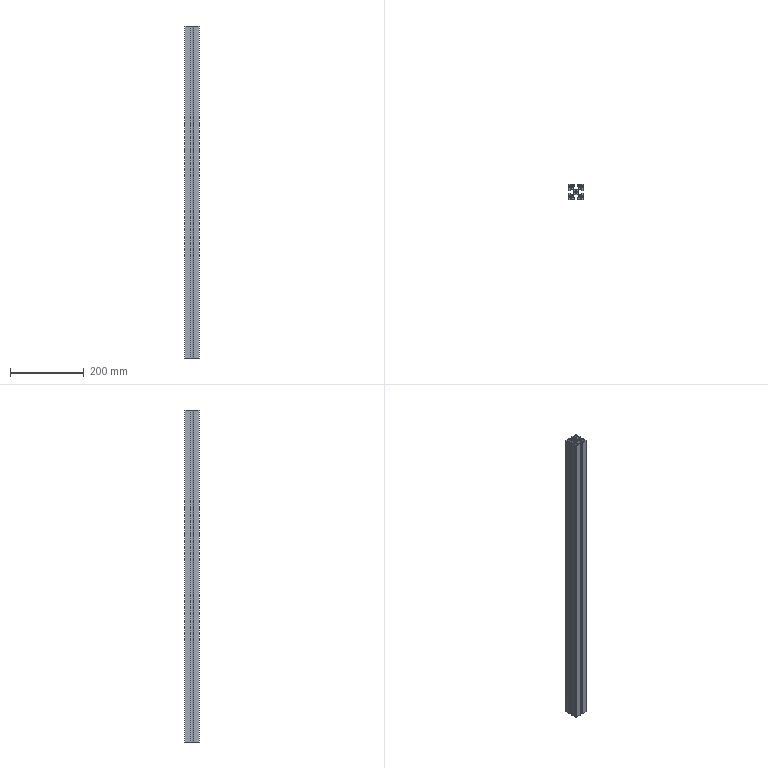Part | STEP file | 09-03 aluminium profile 4040-900 | 1 solid | 53 faces | box 40 x 40 x 900 mm | volume 636225 mm3 | plane 34 | cylinder 19 | commonest cylinder face diameters 8 x8 19 x5 2 x4 6.8 x2